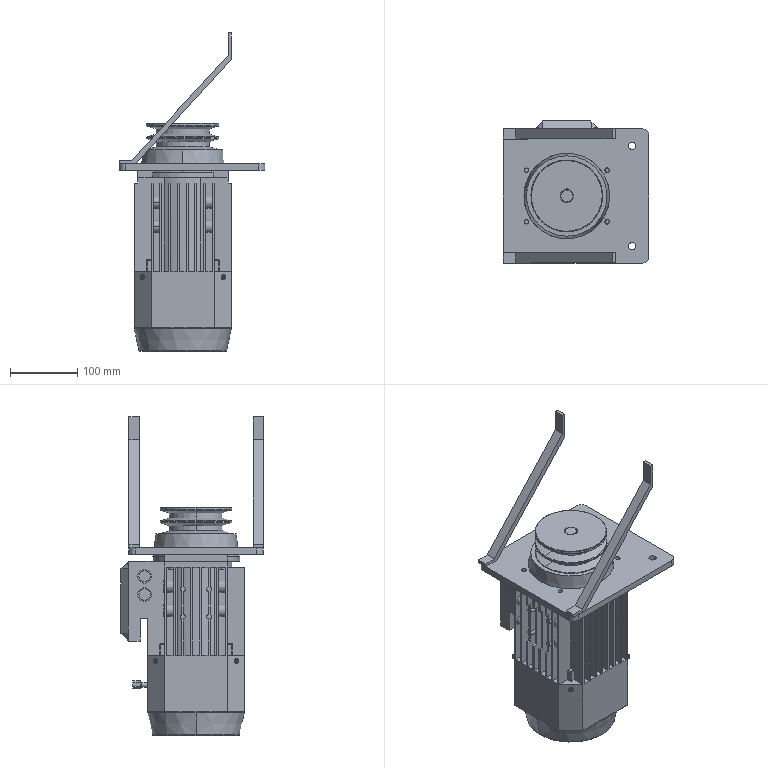Part | SolidWorks | features CompositeCurve 1, MirrorCompFeat 1, ReferencePattern 1 | 5 solids | 1312 faces | box 217.5 x 212 x 474.6 mm | volume 5596236 mm3 | plane 989 | cylinder 221 | spline 82 | cone 20 | commonest cylinder face diameters 108.75 x29 5.8 x24 7.25 x24 2 x20 18 x18 2.32 x12